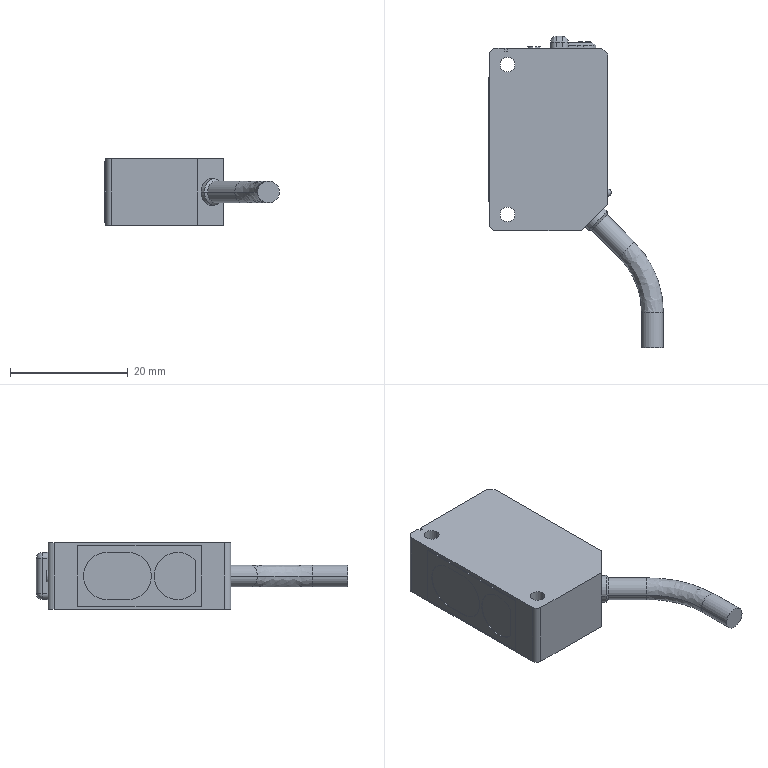Part | STEP file | CX-441 reflective photoelectric sensor 2--50mm_reflective photoelectric sensor441 | 3 solids | 109 faces | box 29.642 x 52.805 x 11.2 mm | volume 7049 mm3 | plane 54 | cylinder 38 | cone 9 | spline 8 | commonest cylinder face diameters 2.05 x11 2 x10 8 x5 2.5 x4 3.7 x4 4 x2